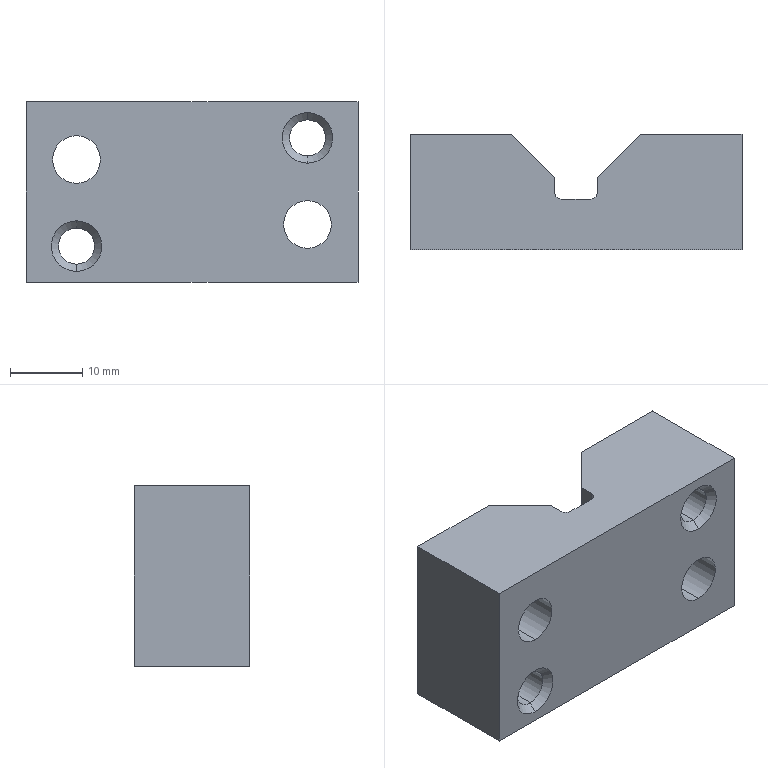Part | SolidWorks | features Chamfer 4, Cut 3, Fillet 2, Extrusion 1 | 1 solid | 36 faces | box 46 x 16 x 25 mm | volume 13455 mm3 | cylinder 14 | plane 14 | cone 8 | commonest cylinder face diameters 5 x4 6.6 x4 12 x4 2 x2
STEP:
#1=CARTESIAN_POINT('',(-16.,-15.,7.5));
#2=VERTEX_POINT('',#1);
#3=CARTESIAN_POINT('',(-16.,-15.,2.5));
#4=VERTEX_POINT('',#3);
#5=CARTESIAN_POINT('',(-16.,-15.,5.));
#6=DIRECTION('',(0.,-1.,0.));
#7=DIRECTION('',(0.,0.,1.));
#8=AXIS2_PLACEMENT_3D('',#5,#6,#7);
#9=CIRCLE('',#8,2.5);
#10=EDGE_CURVE('',#2,#4,#9,.T.);
#11=ORIENTED_EDGE('',*,*,#10,.F.);
#12=CARTESIAN_POINT('',(-16.,-16.,8.5));
#13=VERTEX_POINT('',#12);
#14=CARTESIAN_POINT('',(-16.,-16.,8.5));
#15=DIRECTION('',(0.,-0.7071,0.7071));
#16=VECTOR('',#15,1000.);
#17=LINE('',#14,#16);
#18=EDGE_CURVE('',#2,#13,#17,.T.);
#19=ORIENTED_EDGE('',*,*,#18,.T.);
#20=CARTESIAN_POINT('',(-16.,-16.,1.5));
#21=VERTEX_POINT('',#20);
#22=CARTESIAN_POINT('',(-16.,-16.,5.));
#23=DIRECTION('',(0.,1.,0.));
#24=DIRECTION('',(0.,0.,1.));
#25=AXIS2_PLACEMENT_3D('',#22,#23,#24);
#26=CIRCLE('',#25,3.5);
#27=EDGE_CURVE('',#21,#13,#26,.T.);
#28=ORIENTED_EDGE('',*,*,#27,.F.);
#29=CARTESIAN_POINT('',(-16.,-16.,1.5));
#30=DIRECTION('',(0.,-0.7071,-0.7071));
#31=VECTOR('',#30,1000.);
#32=LINE('',#29,#31);
#33=EDGE_CURVE('',#4,#21,#32,.T.);
#34=ORIENTED_EDGE('',*,*,#33,.F.);
#35=EDGE_LOOP('',(#11,#19,#28,#34));
#36=FACE_OUTER_BOUND('',#35,.T.);
#37=CARTESIAN_POINT('',(-16.,-16.,5.));
#38=DIRECTION('',(0.,-1.,0.));
#39=DIRECTION('',(0.,0.,-1.));
#40=AXIS2_PLACEMENT_3D('',#37,#38,#39);
#41=CONICAL_SURFACE('',#40,3.5,0.7854);
#42=ADVANCED_FACE('',(#36),#41,.F.);
#43=CARTESIAN_POINT('',(16.,-15.,22.5));
#44=VERTEX_POINT('',#43);
#45=CARTESIAN_POINT('',(16.,-15.,17.5));
#46=VERTEX_POINT('',#45);
#47=CARTESIAN_POINT('',(16.,-15.,20.));
#48=DIRECTION('',(0.,-1.,0.));
#49=DIRECTION('',(0.,0.,1.));
#50=AXIS2_PLACEMENT_3D('',#47,#48,#49);
#51=CIRCLE('',#50,2.5);
#52=EDGE_CURVE('',#44,#46,#51,.T.);
#53=ORIENTED_EDGE('',*,*,#52,.F.);
#54=CARTESIAN_POINT('',(16.,-16.,23.5));
#55=VERTEX_POINT('',#54);
#56=CARTESIAN_POINT('',(16.,-16.,23.5));
#57=DIRECTION('',(0.,-0.7071,0.7071));
#58=VECTOR('',#57,1000.);
#59=LINE('',#56,#58);
#60=EDGE_CURVE('',#44,#55,#59,.T.);
#61=ORIENTED_EDGE('',*,*,#60,.T.);
#62=CARTESIAN_POINT('',(16.,-16.,16.5));
#63=VERTEX_POINT('',#62);
#64=CARTESIAN_POINT('',(16.,-16.,20.));
#65=DIRECTION('',(0.,1.,0.));
#66=DIRECTION('',(0.,0.,1.));
#67=AXIS2_PLACEMENT_3D('',#64,#65,#66);
#68=CIRCLE('',#67,3.5);
#69=EDGE_CURVE('',#63,#55,#68,.T.);
#70=ORIENTED_EDGE('',*,*,#69,.F.);
#71=CARTESIAN_POINT('',(16.,-16.,16.5));
#72=DIRECTION('',(0.,-0.7071,-0.7071));
#73=VECTOR('',#72,1000.);
#74=LINE('',#71,#73);
#75=EDGE_CURVE('',#46,#63,#74,.T.);
#76=ORIENTED_EDGE('',*,*,#75,.F.);
#77=EDGE_LOOP('',(#53,#61,#70,#76));
#78=FACE_OUTER_BOUND('',#77,.T.);
#79=CARTESIAN_POINT('',(16.,-16.,20.));
#80=DIRECTION('',(0.,-1.,0.));
#81=DIRECTION('',(0.,0.,-1.));
#82=AXIS2_PLACEMENT_3D('',#79,#80,#81);
#83=CONICAL_SURFACE('',#82,3.5,0.7854);
#84=ADVANCED_FACE('',(#78),#83,.F.);
#85=CARTESIAN_POINT('',(-16.,-1.,2.5));
#86=VERTEX_POINT('',#85);
#87=CARTESIAN_POINT('',(-16.,-1.,7.5));
#88=VERTEX_POINT('',#87);
#89=CARTESIAN_POINT('',(-16.,-1.,5.));
#90=DIRECTION('',(0.,1.,0.));
#91=DIRECTION('',(0.,0.,-1.));
#92=AXIS2_PLACEMENT_3D('',#89,#90,#91);
#93=CIRCLE('',#92,2.5);
#94=EDGE_CURVE('',#86,#88,#93,.T.);
#95=ORIENTED_EDGE('',*,*,#94,.F.);
#96=CARTESIAN_POINT('',(-16.,0.,1.5));
#97=VERTEX_POINT('',#96);
#98=CARTESIAN_POINT('',(-16.,-1.,2.5));
#99=DIRECTION('',(0.,0.7071,-0.7071));
#100=VECTOR('',#99,1000.);
#101=LINE('',#98,#100);
#102=EDGE_CURVE('',#86,#97,#101,.T.);
#103=ORIENTED_EDGE('',*,*,#102,.T.);
#104=CARTESIAN_POINT('',(-16.,0.,8.5));
#105=VERTEX_POINT('',#104);
#106=CARTESIAN_POINT('',(-16.,0.,5.));
#107=DIRECTION('',(0.,-1.,0.));
#108=DIRECTION('',(1.,0.,0.));
#109=AXIS2_PLACEMENT_3D('',#106,#107,#108);
#110=CIRCLE('',#109,3.5);
#111=EDGE_CURVE('',#105,#97,#110,.T.);
#112=ORIENTED_EDGE('',*,*,#111,.F.);
#113=CARTESIAN_POINT('',(-16.,-1.,7.5));
#114=DIRECTION('',(0.,0.7071,0.7071));
#115=VECTOR('',#114,1000.);
#116=LINE('',#113,#115);
#117=EDGE_CURVE('',#88,#105,#116,.T.);
#118=ORIENTED_EDGE('',*,*,#117,.F.);
#119=EDGE_LOOP('',(#95,#103,#112,#118));
#120=FACE_OUTER_BOUND('',#119,.T.);
#121=CARTESIAN_POINT('',(-16.,-1.,5.));
#122=DIRECTION('',(0.,1.,0.));
#123=DIRECTION('',(0.,0.,1.));
#124=AXIS2_PLACEMENT_3D('',#121,#122,#123);
#125=CONICAL_SURFACE('',#124,2.5,0.7854);
#126=ADVANCED_FACE('',(#120),#125,.F.);
#127=CARTESIAN_POINT('',(16.,-1.,17.5));
#128=VERTEX_POINT('',#127);
#129=CARTESIAN_POINT('',(16.,-1.,22.5));
#130=VERTEX_POINT('',#129);
#131=CARTESIAN_POINT('',(16.,-1.,20.));
#132=DIRECTION('',(0.,1.,0.));
#133=DIRECTION('',(0.,0.,-1.));
#134=AXIS2_PLACEMENT_3D('',#131,#132,#133);
#135=CIRCLE('',#134,2.5);
#136=EDGE_CURVE('',#128,#130,#135,.T.);
#137=ORIENTED_EDGE('',*,*,#136,.F.);
#138=CARTESIAN_POINT('',(16.,0.,16.5));
#139=VERTEX_POINT('',#138);
#140=CARTESIAN_POINT('',(16.,-1.,17.5));
#141=DIRECTION('',(0.,0.7071,-0.7071));
#142=VECTOR('',#141,1000.);
#143=LINE('',#140,#142);
#144=EDGE_CURVE('',#128,#139,#143,.T.);
#145=ORIENTED_EDGE('',*,*,#144,.T.);
#146=CARTESIAN_POINT('',(16.,0.,23.5));
#147=VERTEX_POINT('',#146);
#148=CARTESIAN_POINT('',(16.,0.,20.));
#149=DIRECTION('',(0.,-1.,0.));
#150=DIRECTION('',(1.,0.,0.));
#151=AXIS2_PLACEMENT_3D('',#148,#149,#150);
#152=CIRCLE('',#151,3.5);
#153=EDGE_CURVE('',#147,#139,#152,.T.);
#154=ORIENTED_EDGE('',*,*,#153,.F.);
#155=CARTESIAN_POINT('',(16.,-1.,22.5));
#156=DIRECTION('',(0.,0.7071,0.7071));
#157=VECTOR('',#156,1000.);
#158=LINE('',#155,#157);
#159=EDGE_CURVE('',#130,#147,#158,.T.);
#160=ORIENTED_EDGE('',*,*,#159,.F.);
#161=EDGE_LOOP('',(#137,#145,#154,#160));
#162=FACE_OUTER_BOUND('',#161,.T.);
#163=CARTESIAN_POINT('',(16.,-1.,20.));
#164=DIRECTION('',(0.,1.,0.));
#165=DIRECTION('',(0.,0.,1.));
#166=AXIS2_PLACEMENT_3D('',#163,#164,#165);
#167=CONICAL_SURFACE('',#166,2.5,0.7854);
#168=ADVANCED_FACE('',(#162),#167,.F.);
#169=CARTESIAN_POINT('',(16.,-6.,2.));
#170=VERTEX_POINT('',#169);
#171=CARTESIAN_POINT('',(16.,-6.,14.));
#172=VERTEX_POINT('',#171);
#173=CARTESIAN_POINT('',(16.,-6.,8.));
#174=DIRECTION('',(0.,1.,0.));
#175=DIRECTION('',(0.,0.,1.));
#176=AXIS2_PLACEMENT_3D('',#173,#174,#175);
#177=CIRCLE('',#176,6.);
#178=EDGE_CURVE('',#170,#172,#177,.T.);
#179=ORIENTED_EDGE('',*,*,#178,.F.);
#180=CARTESIAN_POINT('',(16.,0.,2.));
#181=VERTEX_POINT('',#180);
#182=CARTESIAN_POINT('',(16.,-6.,2.));
#183=DIRECTION('',(0.,1.,0.));
#184=VECTOR('',#183,1000.);
#185=LINE('',#182,#184);
#186=EDGE_CURVE('',#170,#181,#185,.T.);
#187=ORIENTED_EDGE('',*,*,#186,.T.);
#188=CARTESIAN_POINT('',(16.,0.,14.));
#189=VERTEX_POINT('',#188);
#190=CARTESIAN_POINT('',(16.,0.,8.));
#191=DIRECTION('',(0.,1.,0.));
#192=DIRECTION('',(0.,0.,1.));
#193=AXIS2_PLACEMENT_3D('',#190,#191,#192);
#194=CIRCLE('',#193,6.);
#195=EDGE_CURVE('',#181,#189,#194,.T.);
#196=ORIENTED_EDGE('',*,*,#195,.T.);
#197=CARTESIAN_POINT('',(16.,-6.,14.));
#198=DIRECTION('',(0.,1.,0.));
#199=VECTOR('',#198,1000.);
#200=LINE('',#197,#199);
#201=EDGE_CURVE('',#172,#189,#200,.T.);
#202=ORIENTED_EDGE('',*,*,#201,.F.);
#203=EDGE_LOOP('',(#179,#187,#196,#202));
#204=FACE_OUTER_BOUND('',#203,.T.);
#205=CARTESIAN_POINT('',(16.,-6.,8.));
#206=DIRECTION('',(0.,1.,0.));
#207=DIRECTION('',(0.,0.,1.));
#208=AXIS2_PLACEMENT_3D('',#205,#206,#207);
#209=CYLINDRICAL_SURFACE('',#208,6.);
#210=ADVANCED_FACE('',(#204),#209,.F.);
#211=CARTESIAN_POINT('',(-16.,-6.,11.));
#212=VERTEX_POINT('',#211);
#213=CARTESIAN_POINT('',(-16.,-6.,23.));
#214=VERTEX_POINT('',#213);
#215=CARTESIAN_POINT('',(-16.,-6.,17.));
#216=DIRECTION('',(0.,1.,0.));
#217=DIRECTION('',(0.,0.,1.));
#218=AXIS2_PLACEMENT_3D('',#215,#216,#217);
#219=CIRCLE('',#218,6.);
#220=EDGE_CURVE('',#212,#214,#219,.T.);
#221=ORIENTED_EDGE('',*,*,#220,.F.);
#222=CARTESIAN_POINT('',(-16.,0.,11.));
#223=VERTEX_POINT('',#222);
#224=CARTESIAN_POINT('',(-16.,-6.,11.));
#225=DIRECTION('',(0.,1.,0.));
#226=VECTOR('',#225,1000.);
#227=LINE('',#224,#226);
#228=EDGE_CURVE('',#212,#223,#227,.T.);
#229=ORIENTED_EDGE('',*,*,#228,.T.);
#230=CARTESIAN_POINT('',(-16.,0.,23.));
#231=VERTEX_POINT('',#230);
#232=CARTESIAN_POINT('',(-16.,0.,17.));
#233=DIRECTION('',(0.,1.,0.));
#234=DIRECTION('',(0.,0.,1.));
#235=AXIS2_PLACEMENT_3D('',#232,#233,#234);
#236=CIRCLE('',#235,6.);
#237=EDGE_CURVE('',#223,#231,#236,.T.);
#238=ORIENTED_EDGE('',*,*,#237,.T.);
#239=CARTESIAN_POINT('',(-16.,-6.,23.));
#240=DIRECTION('',(0.,1.,0.));
#241=VECTOR('',#240,1000.);
#242=LINE('',#239,#241);
#243=EDGE_CURVE('',#214,#231,#242,.T.);
#244=ORIENTED_EDGE('',*,*,#243,.F.);
#245=EDGE_LOOP('',(#221,#229,#238,#244));
#246=FACE_OUTER_BOUND('',#245,.T.);
#247=CARTESIAN_POINT('',(-16.,-6.,17.));
#248=DIRECTION('',(0.,1.,0.));
#249=DIRECTION('',(0.,0.,1.));
#250=AXIS2_PLACEMENT_3D('',#247,#248,#249);
#251=CYLINDRICAL_SURFACE('',#250,6.);
#252=ADVANCED_FACE('',(#246),#251,.F.);
#253=ORIENTED_EDGE('',*,*,#52,.T.);
#254=CARTESIAN_POINT('',(16.,-16.,17.5));
#255=DIRECTION('',(0.,1.,0.));
#256=VECTOR('',#255,1000.);
#257=LINE('',#254,#256);
#258=EDGE_CURVE('',#46,#128,#257,.T.);
#259=ORIENTED_EDGE('',*,*,#258,.T.);
#260=ORIENTED_EDGE('',*,*,#136,.T.);
#261=CARTESIAN_POINT('',(16.,-16.,22.5));
#262=DIRECTION('',(0.,1.,0.));
#263=VECTOR('',#262,1000.);
#264=LINE('',#261,#263);
#265=EDGE_CURVE('',#44,#130,#264,.T.);
#266=ORIENTED_EDGE('',*,*,#265,.F.);
#267=EDGE_LOOP('',(#253,#259,#260,#266));
#268=FACE_OUTER_BOUND('',#267,.T.);
#269=CARTESIAN_POINT('',(16.,-16.,20.));
#270=DIRECTION('',(0.,1.,0.));
#271=DIRECTION('',(0.,0.,1.));
#272=AXIS2_PLACEMENT_3D('',#269,#270,#271);
#273=CYLINDRICAL_SURFACE('',#272,2.5);
#274=ADVANCED_FACE('',(#268),#273,.F.);
#275=ORIENTED_EDGE('',*,*,#10,.T.);
#276=CARTESIAN_POINT('',(-16.,-16.,2.5));
#277=DIRECTION('',(0.,1.,0.));
#278=VECTOR('',#277,1000.);
#279=LINE('',#276,#278);
#280=EDGE_CURVE('',#4,#86,#279,.T.);
#281=ORIENTED_EDGE('',*,*,#280,.T.);
#282=ORIENTED_EDGE('',*,*,#94,.T.);
#283=CARTESIAN_POINT('',(-16.,-16.,7.5));
#284=DIRECTION('',(0.,1.,0.));
#285=VECTOR('',#284,1000.);
#286=LINE('',#283,#285);
#287=EDGE_CURVE('',#2,#88,#286,.T.);
#288=ORIENTED_EDGE('',*,*,#287,.F.);
#289=EDGE_LOOP('',(#275,#281,#282,#288));
#290=FACE_OUTER_BOUND('',#289,.T.);
#291=CARTESIAN_POINT('',(-16.,-16.,5.));
#292=DIRECTION('',(0.,1.,0.));
#293=DIRECTION('',(0.,0.,1.));
#294=AXIS2_PLACEMENT_3D('',#291,#292,#293);
#295=CYLINDRICAL_SURFACE('',#294,2.5);
#296=ADVANCED_FACE('',(#290),#295,.F.);
#297=CARTESIAN_POINT('',(-16.,-16.,13.7));
#298=VERTEX_POINT('',#297);
#299=CARTESIAN_POINT('',(-16.,-16.,20.3));
#300=VERTEX_POINT('',#299);
#301=CARTESIAN_POINT('',(-16.,-16.,17.));
#302=DIRECTION('',(0.,1.,0.));
#303=DIRECTION('',(0.,0.,1.));
#304=AXIS2_PLACEMENT_3D('',#301,#302,#303);
#305=CIRCLE('',#304,3.3);
#306=EDGE_CURVE('',#298,#300,#305,.T.);
#307=ORIENTED_EDGE('',*,*,#306,.F.);
#308=CARTESIAN_POINT('',(-16.,-6.,13.7));
#309=VERTEX_POINT('',#308);
#310=CARTESIAN_POINT('',(-16.,-16.,13.7));
#311=DIRECTION('',(0.,1.,0.));
#312=VECTOR('',#311,1000.);
#313=LINE('',#310,#312);
#314=EDGE_CURVE('',#298,#309,#313,.T.);
#315=ORIENTED_EDGE('',*,*,#314,.T.);
#316=CARTESIAN_POINT('',(-16.,-6.,20.3));
#317=VERTEX_POINT('',#316);
#318=CARTESIAN_POINT('',(-16.,-6.,17.));
#319=DIRECTION('',(0.,-1.,0.));
#320=DIRECTION('',(0.,0.,1.));
#321=AXIS2_PLACEMENT_3D('',#318,#319,#320);
#322=CIRCLE('',#321,3.3);
#323=EDGE_CURVE('',#317,#309,#322,.T.);
#324=ORIENTED_EDGE('',*,*,#323,.F.);
#325=CARTESIAN_POINT('',(-16.,-16.,20.3));
#326=DIRECTION('',(0.,1.,0.));
#327=VECTOR('',#326,1000.);
#328=LINE('',#325,#327);
#329=EDGE_CURVE('',#300,#317,#328,.T.);
#330=ORIENTED_EDGE('',*,*,#329,.F.);
#331=EDGE_LOOP('',(#307,#315,#324,#330));
#332=FACE_OUTER_BOUND('',#331,.T.);
#333=CARTESIAN_POINT('',(-16.,-16.,17.));
#334=DIRECTION('',(0.,1.,0.));
#335=DIRECTION('',(0.,0.,1.));
#336=AXIS2_PLACEMENT_3D('',#333,#334,#335);
#337=CYLINDRICAL_SURFACE('',#336,3.3);
#338=ADVANCED_FACE('',(#332),#337,.F.);
#339=CARTESIAN_POINT('',(16.,-16.,4.7));
#340=VERTEX_POINT('',#339);
#341=CARTESIAN_POINT('',(16.,-16.,11.3));
#342=VERTEX_POINT('',#341);
#343=CARTESIAN_POINT('',(16.,-16.,8.));
#344=DIRECTION('',(0.,1.,0.));
#345=DIRECTION('',(0.,0.,1.));
#346=AXIS2_PLACEMENT_3D('',#343,#344,#345);
#347=CIRCLE('',#346,3.3);
#348=EDGE_CURVE('',#340,#342,#347,.T.);
#349=ORIENTED_EDGE('',*,*,#348,.F.);
#350=CARTESIAN_POINT('',(16.,-6.,4.7));
#351=VERTEX_POINT('',#350);
#352=CARTESIAN_POINT('',(16.,-16.,4.7));
#353=DIRECTION('',(0.,1.,0.));
#354=VECTOR('',#353,1000.);
#355=LINE('',#352,#354);
#356=EDGE_CURVE('',#340,#351,#355,.T.);
#357=ORIENTED_EDGE('',*,*,#356,.T.);
#358=CARTESIAN_POINT('',(16.,-6.,11.3));
#359=VERTEX_POINT('',#358);
#360=CARTESIAN_POINT('',(16.,-6.,8.));
#361=DIRECTION('',(0.,-1.,0.));
#362=DIRECTION('',(0.,0.,1.));
#363=AXIS2_PLACEMENT_3D('',#360,#361,#362);
#364=CIRCLE('',#363,3.3);
#365=EDGE_CURVE('',#359,#351,#364,.T.);
#366=ORIENTED_EDGE('',*,*,#365,.F.);
#367=CARTESIAN_POINT('',(16.,-16.,11.3));
#368=DIRECTION('',(0.,1.,0.));
#369=VECTOR('',#368,1000.);
#370=LINE('',#367,#369);
#371=EDGE_CURVE('',#342,#359,#370,.T.);
#372=ORIENTED_EDGE('',*,*,#371,.F.);
#373=EDGE_LOOP('',(#349,#357,#366,#372));
#374=FACE_OUTER_BOUND('',#373,.T.);
#375=CARTESIAN_POINT('',(16.,-16.,8.));
#376=DIRECTION('',(0.,1.,0.));
#377=DIRECTION('',(0.,0.,1.));
#378=AXIS2_PLACEMENT_3D('',#375,#376,#377);
#379=CYLINDRICAL_SURFACE('',#378,3.3);
#380=ADVANCED_FACE('',(#374),#379,.F.);
#381=ORIENTED_EDGE('',*,*,#356,.F.);
#382=CARTESIAN_POINT('',(16.,-16.,8.));
#383=DIRECTION('',(0.,1.,0.));
#384=DIRECTION('',(0.,0.,1.));
#385=AXIS2_PLACEMENT_3D('',#382,#383,#384);
#386=CIRCLE('',#385,3.3);
#387=EDGE_CURVE('',#342,#340,#386,.T.);
#388=ORIENTED_EDGE('',*,*,#387,.F.);
#389=ORIENTED_EDGE('',*,*,#371,.T.);
#390=CARTESIAN_POINT('',(16.,-6.,8.));
#391=DIRECTION('',(0.,-1.,0.));
#392=DIRECTION('',(0.,0.,1.));
#393=AXIS2_PLACEMENT_3D('',#390,#391,#392);
#394=CIRCLE('',#393,3.3);
#395=EDGE_CURVE('',#351,#359,#394,.T.);
#396=ORIENTED_EDGE('',*,*,#395,.F.);
#397=EDGE_LOOP('',(#381,#388,#389,#396));
#398=FACE_OUTER_BOUND('',#397,.T.);
#399=CARTESIAN_POINT('',(16.,-16.,8.));
#400=DIRECTION('',(0.,1.,0.));
#401=DIRECTION('',(0.,0.,1.));
#402=AXIS2_PLACEMENT_3D('',#399,#400,#401);
#403=CYLINDRICAL_SURFACE('',#402,3.3);
#404=ADVANCED_FACE('',(#398),#403,.F.);
#405=ORIENTED_EDGE('',*,*,#314,.F.);
#406=CARTESIAN_POINT('',(-16.,-16.,17.));
#407=DIRECTION('',(0.,1.,0.));
#408=DIRECTION('',(0.,0.,1.));
#409=AXIS2_PLACEMENT_3D('',#406,#407,#408);
#410=CIRCLE('',#409,3.3);
#411=EDGE_CURVE('',#300,#298,#410,.T.);
#412=ORIENTED_EDGE('',*,*,#411,.F.);
#413=ORIENTED_EDGE('',*,*,#329,.T.);
#414=CARTESIAN_POINT('',(-16.,-6.,17.));
#415=DIRECTION('',(0.,-1.,0.));
#416=DIRECTION('',(0.,0.,1.));
#417=AXIS2_PLACEMENT_3D('',#414,#415,#416);
#418=CIRCLE('',#417,3.3);
#419=EDGE_CURVE('',#309,#317,#418,.T.);
#420=ORIENTED_EDGE('',*,*,#419,.F.);
#421=EDGE_LOOP('',(#405,#412,#413,#420));
#422=FACE_OUTER_BOUND('',#421,.T.);
#423=CARTESIAN_POINT('',(-16.,-16.,17.));
#424=DIRECTION('',(0.,1.,0.));
#425=DIRECTION('',(0.,0.,1.));
#426=AXIS2_PLACEMENT_3D('',#423,#424,#425);
#427=CYLINDRICAL_SURFACE('',#426,3.3);
#428=ADVANCED_FACE('',(#422),#427,.F.);
#429=ORIENTED_EDGE('',*,*,#111,.T.);
#430=CARTESIAN_POINT('',(-16.,0.,5.));
#431=DIRECTION('',(0.,-1.,0.));
#432=DIRECTION('',(1.,0.,0.));
#433=AXIS2_PLACEMENT_3D('',#430,#431,#432);
#434=CIRCLE('',#433,3.5);
#435=EDGE_CURVE('',#97,#105,#434,.T.);
#436=ORIENTED_EDGE('',*,*,#435,.T.);
#437=EDGE_LOOP('',(#429,#436));
#438=FACE_BOUND('',#437,.T.);
#439=CARTESIAN_POINT('',(-16.,0.,17.));
#440=DIRECTION('',(0.,1.,0.));
#441=DIRECTION('',(0.,0.,1.));
#442=AXIS2_PLACEMENT_3D('',#439,#440,#441);
#443=CIRCLE('',#442,6.);
#444=EDGE_CURVE('',#231,#223,#443,.T.);
#445=ORIENTED_EDGE('',*,*,#444,.F.);
#446=ORIENTED_EDGE('',*,*,#237,.F.);
#447=EDGE_LOOP('',(#445,#446));
#448=FACE_BOUND('',#447,.T.);
#449=CARTESIAN_POINT('',(-9.,0.,25.));
#450=VERTEX_POINT('',#449);
#451=CARTESIAN_POINT('',(-23.,0.,25.));
#452=VERTEX_POINT('',#451);
#453=CARTESIAN_POINT('',(-23.,0.,25.));
#454=DIRECTION('',(-1.,0.,0.));
#455=VECTOR('',#454,1000.);
#456=LINE('',#453,#455);
#457=EDGE_CURVE('',#450,#452,#456,.T.);
#458=ORIENTED_EDGE('',*,*,#457,.F.);
#459=CARTESIAN_POINT('',(-9.,0.,0.));
#460=VERTEX_POINT('',#459);
#461=CARTESIAN_POINT('',(-9.,0.,0.));
#462=DIRECTION('',(0.,0.,1.));
#463=VECTOR('',#462,1000.);
#464=LINE('',#461,#463);
#465=EDGE_CURVE('',#460,#450,#464,.T.);
#466=ORIENTED_EDGE('',*,*,#465,.F.);
#467=CARTESIAN_POINT('',(-23.,0.,0.));
#468=VERTEX_POINT('',#467);
#469=CARTESIAN_POINT('',(-23.,0.,0.));
#470=DIRECTION('',(-1.,0.,0.));
#471=VECTOR('',#470,1000.);
#472=LINE('',#469,#471);
#473=EDGE_CURVE('',#460,#468,#472,.T.);
#474=ORIENTED_EDGE('',*,*,#473,.T.);
#475=CARTESIAN_POINT('',(-23.,0.,25.));
#476=DIRECTION('',(0.,0.,-1.));
#477=VECTOR('',#476,1000.);
#478=LINE('',#475,#477);
#479=EDGE_CURVE('',#452,#468,#478,.T.);
#480=ORIENTED_EDGE('',*,*,#479,.F.);
#481=EDGE_LOOP('',(#458,#466,#474,#480));
#482=FACE_OUTER_BOUND('',#481,.T.);
#483=CARTESIAN_POINT('',(-23.,0.,25.));
#484=DIRECTION('',(0.,-1.,0.));
#485=DIRECTION('',(1.,0.,0.));
#486=AXIS2_PLACEMENT_3D('',#483,#484,#485);
#487=PLANE('',#486);
#488=ADVANCED_FACE('',(#438,#448,#482),#487,.F.);
#489=CARTESIAN_POINT('',(-23.,-16.,0.));
#490=VERTEX_POINT('',#489);
#491=CARTESIAN_POINT('',(-23.,0.,0.));
#492=DIRECTION('',(0.,-1.,0.));
#493=VECTOR('',#492,1000.);
#494=LINE('',#491,#493);
#495=EDGE_CURVE('',#468,#490,#494,.T.);
#496=ORIENTED_EDGE('',*,*,#495,.T.);
#497=CARTESIAN_POINT('',(-23.,-16.,25.));
#498=VERTEX_POINT('',#497);
#499=CARTESIAN_POINT('',(-23.,-16.,25.));
#500=DIRECTION('',(0.,0.,-1.));
#501=VECTOR('',#500,1000.);
#502=LINE('',#499,#501);
#503=EDGE_CURVE('',#498,#490,#502,.T.);
#504=ORIENTED_EDGE('',*,*,#503,.F.);
#505=CARTESIAN_POINT('',(-23.,0.,25.));
#506=DIRECTION('',(0.,-1.,0.));
#507=VECTOR('',#506,1000.);
#508=LINE('',#505,#507);
#509=EDGE_CURVE('',#452,#498,#508,.T.);
#510=ORIENTED_EDGE('',*,*,#509,.F.);
#511=ORIENTED_EDGE('',*,*,#479,.T.);
#512=EDGE_LOOP('',(#496,#504,#510,#511));
#513=FACE_OUTER_BOUND('',#512,.T.);
#514=CARTESIAN_POINT('',(-23.,0.,25.));
#515=DIRECTION('',(1.,0.,0.));
#516=DIRECTION('',(0.,1.,0.));
#517=AXIS2_PLACEMENT_3D('',#514,#515,#516);
#518=PLANE('',#517);
#519=ADVANCED_FACE('',(#513),#518,.F.);
#520=ORIENTED_EDGE('',*,*,#27,.T.);
#521=CARTESIAN_POINT('',(-16.,-16.,5.));
#522=DIRECTION('',(0.,1.,0.));
#523=DIRECTION('',(0.,0.,1.));
#524=AXIS2_PLACEMENT_3D('',#521,#522,#523);
#525=CIRCLE('',#524,3.5);
#526=EDGE_CURVE('',#13,#21,#525,.T.);
#527=ORIENTED_EDGE('',*,*,#526,.T.);
#528=EDGE_LOOP('',(#520,#527));
#529=FACE_BOUND('',#528,.T.);
#530=ORIENTED_EDGE('',*,*,#69,.T.);
#531=CARTESIAN_POINT('',(16.,-16.,20.));
#532=DIRECTION('',(0.,1.,0.));
#533=DIRECTION('',(0.,0.,1.));
#534=AXIS2_PLACEMENT_3D('',#531,#532,#533);
#535=CIRCLE('',#534,3.5);
#536=EDGE_CURVE('',#55,#63,#535,.T.);
#537=ORIENTED_EDGE('',*,*,#536,.T.);
#538=EDGE_LOOP('',(#530,#537));
#539=FACE_BOUND('',#538,.T.);
#540=ORIENTED_EDGE('',*,*,#387,.T.);
#541=ORIENTED_EDGE('',*,*,#348,.T.);
#542=EDGE_LOOP('',(#540,#541));
#543=FACE_BOUND('',#542,.T.);
#544=ORIENTED_EDGE('',*,*,#411,.T.);
#545=ORIENTED_EDGE('',*,*,#306,.T.);
#546=EDGE_LOOP('',(#544,#545));
#547=FACE_BOUND('',#546,.T.);
#548=CARTESIAN_POINT('',(23.,-16.,0.));
#549=VERTEX_POINT('',#548);
#550=CARTESIAN_POINT('',(-23.,-16.,0.));
#551=DIRECTION('',(1.,0.,0.));
#552=VECTOR('',#551,1000.);
#553=LINE('',#550,#552);
#554=EDGE_CURVE('',#490,#549,#553,.T.);
#555=ORIENTED_EDGE('',*,*,#554,.T.);
#556=CARTESIAN_POINT('',(23.,-16.,25.));
#557=VERTEX_POINT('',#556);
#558=CARTESIAN_POINT('',(23.,-16.,25.));
#559=DIRECTION('',(0.,0.,-1.));
#560=VECTOR('',#559,1000.);
#561=LINE('',#558,#560);
#562=EDGE_CURVE('',#557,#549,#561,.T.);
#563=ORIENTED_EDGE('',*,*,#562,.F.);
#564=CARTESIAN_POINT('',(-23.,-16.,25.));
#565=DIRECTION('',(1.,0.,0.));
#566=VECTOR('',#565,1000.);
#567=LINE('',#564,#566);
#568=EDGE_CURVE('',#498,#557,#567,.T.);
#569=ORIENTED_EDGE('',*,*,#568,.F.);
#570=ORIENTED_EDGE('',*,*,#503,.T.);
#571=EDGE_LOOP('',(#555,#563,#569,#570));
#572=FACE_OUTER_BOUND('',#571,.T.);
#573=CARTESIAN_POINT('',(-23.,-16.,25.));
#574=DIRECTION('',(0.,1.,0.));
#575=DIRECTION('',(0.,0.,1.));
#576=AXIS2_PLACEMENT_3D('',#573,#574,#575);
#577=PLANE('',#576);
#578=ADVANCED_FACE('',(#529,#539,#543,#547,#572),#577,.F.);
#579=CARTESIAN_POINT('',(23.,0.,0.));
#580=VERTEX_POINT('',#579);
#581=CARTESIAN_POINT('',(23.,0.,0.));
#582=DIRECTION('',(0.,1.,0.));
#583=VECTOR('',#582,1000.);
#584=LINE('',#581,#583);
#585=EDGE_CURVE('',#549,#580,#584,.T.);
#586=ORIENTED_EDGE('',*,*,#585,.T.);
#587=CARTESIAN_POINT('',(23.,0.,25.));
#588=VERTEX_POINT('',#587);
#589=CARTESIAN_POINT('',(23.,0.,25.));
#590=DIRECTION('',(0.,0.,-1.));
#591=VECTOR('',#590,1000.);
#592=LINE('',#589,#591);
#593=EDGE_CURVE('',#588,#580,#592,.T.);
#594=ORIENTED_EDGE('',*,*,#593,.F.);
#595=CARTESIAN_POINT('',(23.,0.,25.));
#596=DIRECTION('',(0.,1.,0.));
#597=VECTOR('',#596,1000.);
#598=LINE('',#595,#597);
#599=EDGE_CURVE('',#557,#588,#598,.T.);
#600=ORIENTED_EDGE('',*,*,#599,.F.);
#601=ORIENTED_EDGE('',*,*,#562,.T.);
#602=EDGE_LOOP('',(#586,#594,#600,#601));
#603=FACE_OUTER_BOUND('',#602,.T.);
#604=CARTESIAN_POINT('',(23.,0.,25.));
#605=DIRECTION('',(-1.,0.,0.));
#606=DIRECTION('',(0.,-1.,0.));
#607=AXIS2_PLACEMENT_3D('',#604,#605,#606);
#608=PLANE('',#607);
#609=ADVANCED_FACE('',(#603),#608,.F.);
#610=ORIENTED_EDGE('',*,*,#153,.T.);
#611=CARTESIAN_POINT('',(16.,0.,20.));
#612=DIRECTION('',(0.,-1.,0.));
#613=DIRECTION('',(1.,0.,0.));
#614=AXIS2_PLACEMENT_3D('',#611,#612,#613);
#615=CIRCLE('',#614,3.5);
#616=EDGE_CURVE('',#139,#147,#615,.T.);
#617=ORIENTED_EDGE('',*,*,#616,.T.);
#618=EDGE_LOOP('',(#610,#617));
#619=FACE_BOUND('',#618,.T.);
#620=CARTESIAN_POINT('',(16.,0.,8.));
#621=DIRECTION('',(0.,1.,0.));
#622=DIRECTION('',(0.,0.,1.));
#623=AXIS2_PLACEMENT_3D('',#620,#621,#622);
#624=CIRCLE('',#623,6.);
#625=EDGE_CURVE('',#189,#181,#624,.T.);
#626=ORIENTED_EDGE('',*,*,#625,.F.);
#627=ORIENTED_EDGE('',*,*,#195,.F.);
#628=EDGE_LOOP('',(#626,#627));
#629=FACE_BOUND('',#628,.T.);
#630=CARTESIAN_POINT('',(9.,0.,0.));
#631=VERTEX_POINT('',#630);
#632=CARTESIAN_POINT('',(-23.,0.,0.));
#633=DIRECTION('',(-1.,0.,0.));
#634=VECTOR('',#633,1000.);
#635=LINE('',#632,#634);
#636=EDGE_CURVE('',#580,#631,#635,.T.);
#637=ORIENTED_EDGE('',*,*,#636,.T.);
#638=CARTESIAN_POINT('',(9.,0.,25.));
#639=VERTEX_POINT('',#638);
#640=CARTESIAN_POINT('',(9.,0.,0.));
#641=DIRECTION('',(0.,0.,1.));
#642=VECTOR('',#641,1000.);
#643=LINE('',#640,#642);
#644=EDGE_CURVE('',#631,#639,#643,.T.);
#645=ORIENTED_EDGE('',*,*,#644,.T.);
#646=CARTESIAN_POINT('',(-23.,0.,25.));
#647=DIRECTION('',(-1.,0.,0.));
#648=VECTOR('',#647,1000.);
#649=LINE('',#646,#648);
#650=EDGE_CURVE('',#588,#639,#649,.T.);
#651=ORIENTED_EDGE('',*,*,#650,.F.);
#652=ORIENTED_EDGE('',*,*,#593,.T.);
#653=EDGE_LOOP('',(#637,#645,#651,#652));
#654=FACE_OUTER_BOUND('',#653,.T.);
#655=CARTESIAN_POINT('',(-23.,0.,25.));
#656=DIRECTION('',(0.,-1.,0.));
#657=DIRECTION('',(1.,0.,0.));
#658=AXIS2_PLACEMENT_3D('',#655,#656,#657);
#659=PLANE('',#658);
#660=ADVANCED_FACE('',(#619,#629,#654),#659,.F.);
#661=CARTESIAN_POINT('',(-3.,-6.,25.));
#662=VERTEX_POINT('',#661);
#663=CARTESIAN_POINT('',(-9.,0.,25.));
#664=DIRECTION('',(0.7071,-0.7071,0.));
#665=VECTOR('',#664,1000.);
#666=LINE('',#663,#665);
#667=EDGE_CURVE('',#450,#662,#666,.T.);
#668=ORIENTED_EDGE('',*,*,#667,.F.);
#669=ORIENTED_EDGE('',*,*,#457,.T.);
#670=ORIENTED_EDGE('',*,*,#509,.T.);
#671=ORIENTED_EDGE('',*,*,#568,.T.);
#672=ORIENTED_EDGE('',*,*,#599,.T.);
#673=ORIENTED_EDGE('',*,*,#650,.T.);
#674=CARTESIAN_POINT('',(3.,-6.,25.));
#675=VERTEX_POINT('',#674);
#676=CARTESIAN_POINT('',(9.,0.,25.));
#677=DIRECTION('',(0.7071,0.7071,0.));
#678=VECTOR('',#677,1000.);
#679=LINE('',#676,#678);
#680=EDGE_CURVE('',#675,#639,#679,.T.);
#681=ORIENTED_EDGE('',*,*,#680,.F.);
#682=CARTESIAN_POINT('',(3.,-8.,25.));
#683=VERTEX_POINT('',#682);
#684=CARTESIAN_POINT('',(3.,-6.,25.));
#685=DIRECTION('',(0.,1.,0.));
#686=VECTOR('',#685,1000.);
#687=LINE('',#684,#686);
#688=EDGE_CURVE('',#683,#675,#687,.T.);
#689=ORIENTED_EDGE('',*,*,#688,.F.);
#690=CARTESIAN_POINT('',(2.,-9.,25.));
#691=VERTEX_POINT('',#690);
#692=CARTESIAN_POINT('',(2.,-8.,25.));
#693=DIRECTION('',(0.,0.,-1.));
#694=DIRECTION('',(1.,0.,0.));
#695=AXIS2_PLACEMENT_3D('',#692,#693,#694);
#696=CIRCLE('',#695,1.);
#697=EDGE_CURVE('',#683,#691,#696,.T.);
#698=ORIENTED_EDGE('',*,*,#697,.T.);
#699=CARTESIAN_POINT('',(-2.,-9.,25.));
#700=VERTEX_POINT('',#699);
#701=CARTESIAN_POINT('',(-3.,-9.,25.));
#702=DIRECTION('',(1.,0.,0.));
#703=VECTOR('',#702,1000.);
#704=LINE('',#701,#703);
#705=EDGE_CURVE('',#700,#691,#704,.T.);
#706=ORIENTED_EDGE('',*,*,#705,.F.);
#707=CARTESIAN_POINT('',(-3.,-8.,25.));
#708=VERTEX_POINT('',#707);
#709=CARTESIAN_POINT('',(-2.,-8.,25.));
#710=DIRECTION('',(0.,0.,-1.));
#711=DIRECTION('',(1.,0.,0.));
#712=AXIS2_PLACEMENT_3D('',#709,#710,#711);
#713=CIRCLE('',#712,1.);
#714=EDGE_CURVE('',#700,#708,#713,.T.);
#715=ORIENTED_EDGE('',*,*,#714,.T.);
#716=CARTESIAN_POINT('',(-3.,-6.,25.));
#717=DIRECTION('',(0.,-1.,0.));
#718=VECTOR('',#717,1000.);
#719=LINE('',#716,#718);
#720=EDGE_CURVE('',#662,#708,#719,.T.);
#721=ORIENTED_EDGE('',*,*,#720,.F.);
#722=EDGE_LOOP('',(#668,#669,#670,#671,#672,#673,#681,#689,#698,#706,#715,#721));
#723=FACE_OUTER_BOUND('',#722,.T.);
#724=CARTESIAN_POINT('',(-23.,0.,25.));
#725=DIRECTION('',(0.,0.,1.));
#726=DIRECTION('',(1.,0.,0.));
#727=AXIS2_PLACEMENT_3D('',#724,#725,#726);
#728=PLANE('',#727);
#729=ADVANCED_FACE('',(#723),#728,.T.);
#730=ORIENTED_EDGE('',*,*,#473,.F.);
#731=CARTESIAN_POINT('',(-3.,-6.,0.));
#732=VERTEX_POINT('',#731);
#733=CARTESIAN_POINT('',(-9.,0.,0.));
#734=DIRECTION('',(0.7071,-0.7071,0.));
#735=VECTOR('',#734,1000.);
#736=LINE('',#733,#735);
#737=EDGE_CURVE('',#460,#732,#736,.T.);
#738=ORIENTED_EDGE('',*,*,#737,.T.);
#739=CARTESIAN_POINT('',(-3.,-8.,0.));
#740=VERTEX_POINT('',#739);
#741=CARTESIAN_POINT('',(-3.,-6.,0.));
#742=DIRECTION('',(0.,-1.,0.));
#743=VECTOR('',#742,1000.);
#744=LINE('',#741,#743);
#745=EDGE_CURVE('',#732,#740,#744,.T.);
#746=ORIENTED_EDGE('',*,*,#745,.T.);
#747=CARTESIAN_POINT('',(-2.,-9.,0.));
#748=VERTEX_POINT('',#747);
#749=CARTESIAN_POINT('',(-2.,-8.,0.));
#750=DIRECTION('',(0.,0.,1.));
#751=DIRECTION('',(1.,0.,0.));
#752=AXIS2_PLACEMENT_3D('',#749,#750,#751);
#753=CIRCLE('',#752,1.);
#754=EDGE_CURVE('',#740,#748,#753,.T.);
#755=ORIENTED_EDGE('',*,*,#754,.T.);
#756=CARTESIAN_POINT('',(2.,-9.,0.));
#757=VERTEX_POINT('',#756);
#758=CARTESIAN_POINT('',(-3.,-9.,0.));
#759=DIRECTION('',(1.,0.,0.));
#760=VECTOR('',#759,1000.);
#761=LINE('',#758,#760);
#762=EDGE_CURVE('',#748,#757,#761,.T.);
#763=ORIENTED_EDGE('',*,*,#762,.T.);
#764=CARTESIAN_POINT('',(3.,-8.,0.));
#765=VERTEX_POINT('',#764);
#766=CARTESIAN_POINT('',(2.,-8.,0.));
#767=DIRECTION('',(0.,0.,1.));
#768=DIRECTION('',(1.,0.,0.));
#769=AXIS2_PLACEMENT_3D('',#766,#767,#768);
#770=CIRCLE('',#769,1.);
#771=EDGE_CURVE('',#757,#765,#770,.T.);
#772=ORIENTED_EDGE('',*,*,#771,.T.);
#773=CARTESIAN_POINT('',(3.,-6.,0.));
#774=VERTEX_POINT('',#773);
#775=CARTESIAN_POINT('',(3.,-6.,0.));
#776=DIRECTION('',(0.,1.,0.));
#777=VECTOR('',#776,1000.);
#778=LINE('',#775,#777);
#779=EDGE_CURVE('',#765,#774,#778,.T.);
#780=ORIENTED_EDGE('',*,*,#779,.T.);
#781=CARTESIAN_POINT('',(9.,0.,0.));
#782=DIRECTION('',(0.7071,0.7071,0.));
#783=VECTOR('',#782,1000.);
#784=LINE('',#781,#783);
#785=EDGE_CURVE('',#774,#631,#784,.T.);
#786=ORIENTED_EDGE('',*,*,#785,.T.);
#787=ORIENTED_EDGE('',*,*,#636,.F.);
#788=ORIENTED_EDGE('',*,*,#585,.F.);
#789=ORIENTED_EDGE('',*,*,#554,.F.);
#790=ORIENTED_EDGE('',*,*,#495,.F.);
#791=EDGE_LOOP('',(#730,#738,#746,#755,#763,#772,#780,#786,#787,#788,#789,#790));
#792=FACE_OUTER_BOUND('',#791,.T.);
#793=CARTESIAN_POINT('',(-23.,0.,0.));
#794=DIRECTION('',(0.,0.,1.));
#795=DIRECTION('',(1.,0.,0.));
#796=AXIS2_PLACEMENT_3D('',#793,#794,#795);
#797=PLANE('',#796);
#798=ADVANCED_FACE('',(#792),#797,.F.);
#799=ORIENTED_EDGE('',*,*,#720,.T.);
#800=CARTESIAN_POINT('',(-3.,-8.,0.));
#801=DIRECTION('',(0.,0.,-1.));
#802=VECTOR('',#801,1000.);
#803=LINE('',#800,#802);
#804=EDGE_CURVE('',#708,#740,#803,.T.);
#805=ORIENTED_EDGE('',*,*,#804,.T.);
#806=ORIENTED_EDGE('',*,*,#745,.F.);
#807=CARTESIAN_POINT('',(-3.,-6.,0.));
#808=DIRECTION('',(0.,0.,1.));
#809=VECTOR('',#808,1000.);
#810=LINE('',#807,#809);
#811=EDGE_CURVE('',#732,#662,#810,.T.);
#812=ORIENTED_EDGE('',*,*,#811,.T.);
#813=EDGE_LOOP('',(#799,#805,#806,#812));
#814=FACE_OUTER_BOUND('',#813,.T.);
#815=CARTESIAN_POINT('',(-3.,-6.,0.));
#816=DIRECTION('',(-1.,0.,0.));
#817=DIRECTION('',(0.,0.,1.));
#818=AXIS2_PLACEMENT_3D('',#815,#816,#817);
#819=PLANE('',#818);
#820=ADVANCED_FACE('',(#814),#819,.F.);
#821=ORIENTED_EDGE('',*,*,#667,.T.);
#822=ORIENTED_EDGE('',*,*,#811,.F.);
#823=ORIENTED_EDGE('',*,*,#737,.F.);
#824=ORIENTED_EDGE('',*,*,#465,.T.);
#825=EDGE_LOOP('',(#821,#822,#823,#824));
#826=FACE_OUTER_BOUND('',#825,.T.);
#827=CARTESIAN_POINT('',(-9.,0.,0.));
#828=DIRECTION('',(-0.7071,-0.7071,0.));
#829=DIRECTION('',(0.7071,-0.7071,0.));
#830=AXIS2_PLACEMENT_3D('',#827,#828,#829);
#831=PLANE('',#830);
#832=ADVANCED_FACE('',(#826),#831,.F.);
#833=ORIENTED_EDGE('',*,*,#680,.T.);
#834=ORIENTED_EDGE('',*,*,#644,.F.);
#835=ORIENTED_EDGE('',*,*,#785,.F.);
#836=CARTESIAN_POINT('',(3.,-6.,0.));
#837=DIRECTION('',(0.,0.,1.));
#838=VECTOR('',#837,1000.);
#839=LINE('',#836,#838);
#840=EDGE_CURVE('',#774,#675,#839,.T.);
#841=ORIENTED_EDGE('',*,*,#840,.T.);
#842=EDGE_LOOP('',(#833,#834,#835,#841));
#843=FACE_OUTER_BOUND('',#842,.T.);
#844=CARTESIAN_POINT('',(9.,0.,0.));
#845=DIRECTION('',(0.7071,-0.7071,0.));
#846=DIRECTION('',(0.7071,0.7071,0.));
#847=AXIS2_PLACEMENT_3D('',#844,#845,#846);
#848=PLANE('',#847);
#849=ADVANCED_FACE('',(#843),#848,.F.);
#850=ORIENTED_EDGE('',*,*,#779,.F.);
#851=CARTESIAN_POINT('',(3.,-8.,25.));
#852=DIRECTION('',(0.,0.,1.));
#853=VECTOR('',#852,1000.);
#854=LINE('',#851,#853);
#855=EDGE_CURVE('',#765,#683,#854,.T.);
#856=ORIENTED_EDGE('',*,*,#855,.T.);
#857=ORIENTED_EDGE('',*,*,#688,.T.);
#858=ORIENTED_EDGE('',*,*,#840,.F.);
#859=EDGE_LOOP('',(#850,#856,#857,#858));
#860=FACE_OUTER_BOUND('',#859,.T.);
#861=CARTESIAN_POINT('',(3.,-6.,0.));
#862=DIRECTION('',(1.,0.,0.));
#863=DIRECTION('',(0.,1.,0.));
#864=AXIS2_PLACEMENT_3D('',#861,#862,#863);
#865=PLANE('',#864);
#866=ADVANCED_FACE('',(#860),#865,.F.);
#867=ORIENTED_EDGE('',*,*,#705,.T.);
#868=CARTESIAN_POINT('',(2.,-9.,0.));
#869=DIRECTION('',(0.,0.,-1.));
#870=VECTOR('',#869,1000.);
#871=LINE('',#868,#870);
#872=EDGE_CURVE('',#691,#757,#871,.T.);
#873=ORIENTED_EDGE('',*,*,#872,.T.);
#874=ORIENTED_EDGE('',*,*,#762,.F.);
#875=CARTESIAN_POINT('',(-2.,-9.,25.));
#876=DIRECTION('',(0.,0.,1.));
#877=VECTOR('',#876,1000.);
#878=LINE('',#875,#877);
#879=EDGE_CURVE('',#748,#700,#878,.T.);
#880=ORIENTED_EDGE('',*,*,#879,.T.);
#881=EDGE_LOOP('',(#867,#873,#874,#880));
#882=FACE_OUTER_BOUND('',#881,.T.);
#883=CARTESIAN_POINT('',(-3.,-9.,0.));
#884=DIRECTION('',(0.,-1.,0.));
#885=DIRECTION('',(0.,0.,-1.));
#886=AXIS2_PLACEMENT_3D('',#883,#884,#885);
#887=PLANE('',#886);
#888=ADVANCED_FACE('',(#882),#887,.F.);
#889=ORIENTED_EDGE('',*,*,#754,.F.);
#890=ORIENTED_EDGE('',*,*,#804,.F.);
#891=ORIENTED_EDGE('',*,*,#714,.F.);
#892=ORIENTED_EDGE('',*,*,#879,.F.);
#893=EDGE_LOOP('',(#889,#890,#891,#892));
#894=FACE_OUTER_BOUND('',#893,.T.);
#895=CARTESIAN_POINT('',(-2.,-8.,0.));
#896=DIRECTION('',(0.,0.,-1.));
#897=DIRECTION('',(-1.,0.,0.));
#898=AXIS2_PLACEMENT_3D('',#895,#896,#897);
#899=CYLINDRICAL_SURFACE('',#898,1.);
#900=ADVANCED_FACE('',(#894),#899,.F.);
#901=ORIENTED_EDGE('',*,*,#771,.F.);
#902=ORIENTED_EDGE('',*,*,#872,.F.);
#903=ORIENTED_EDGE('',*,*,#697,.F.);
#904=ORIENTED_EDGE('',*,*,#855,.F.);
#905=EDGE_LOOP('',(#901,#902,#903,#904));
#906=FACE_OUTER_BOUND('',#905,.T.);
#907=CARTESIAN_POINT('',(2.,-8.,0.));
#908=DIRECTION('',(0.,0.,-1.));
#909=DIRECTION('',(-1.,0.,0.));
#910=AXIS2_PLACEMENT_3D('',#907,#908,#909);
#911=CYLINDRICAL_SURFACE('',#910,1.);
#912=ADVANCED_FACE('',(#906),#911,.F.);
#913=ORIENTED_EDGE('',*,*,#280,.F.);
#914=CARTESIAN_POINT('',(-16.,-15.,5.));
#915=DIRECTION('',(0.,-1.,0.));
#916=DIRECTION('',(0.,0.,1.));
#917=AXIS2_PLACEMENT_3D('',#914,#915,#916);
#918=CIRCLE('',#917,2.5);
#919=EDGE_CURVE('',#4,#2,#918,.T.);
#920=ORIENTED_EDGE('',*,*,#919,.T.);
#921=ORIENTED_EDGE('',*,*,#287,.T.);
#922=CARTESIAN_POINT('',(-16.,-1.,5.));
#923=DIRECTION('',(0.,1.,0.));
#924=DIRECTION('',(0.,0.,-1.));
#925=AXIS2_PLACEMENT_3D('',#922,#923,#924);
#926=CIRCLE('',#925,2.5);
#927=EDGE_CURVE('',#88,#86,#926,.T.);
#928=ORIENTED_EDGE('',*,*,#927,.T.);
#929=EDGE_LOOP('',(#913,#920,#921,#928));
#930=FACE_OUTER_BOUND('',#929,.T.);
#931=CARTESIAN_POINT('',(-16.,-16.,5.));
#932=DIRECTION('',(0.,1.,0.));
#933=DIRECTION('',(0.,0.,1.));
#934=AXIS2_PLACEMENT_3D('',#931,#932,#933);
#935=CYLINDRICAL_SURFACE('',#934,2.5);
#936=ADVANCED_FACE('',(#930),#935,.F.);
#937=ORIENTED_EDGE('',*,*,#258,.F.);
#938=CARTESIAN_POINT('',(16.,-15.,20.));
#939=DIRECTION('',(0.,-1.,0.));
#940=DIRECTION('',(0.,0.,1.));
#941=AXIS2_PLACEMENT_3D('',#938,#939,#940);
#942=CIRCLE('',#941,2.5);
#943=EDGE_CURVE('',#46,#44,#942,.T.);
#944=ORIENTED_EDGE('',*,*,#943,.T.);
#945=ORIENTED_EDGE('',*,*,#265,.T.);
#946=CARTESIAN_POINT('',(16.,-1.,20.));
#947=DIRECTION('',(0.,1.,0.));
#948=DIRECTION('',(0.,0.,-1.));
#949=AXIS2_PLACEMENT_3D('',#946,#947,#948);
#950=CIRCLE('',#949,2.5);
#951=EDGE_CURVE('',#130,#128,#950,.T.);
#952=ORIENTED_EDGE('',*,*,#951,.T.);
#953=EDGE_LOOP('',(#937,#944,#945,#952));
#954=FACE_OUTER_BOUND('',#953,.T.);
#955=CARTESIAN_POINT('',(16.,-16.,20.));
#956=DIRECTION('',(0.,1.,0.));
#957=DIRECTION('',(0.,0.,1.));
#958=AXIS2_PLACEMENT_3D('',#955,#956,#957);
#959=CYLINDRICAL_SURFACE('',#958,2.5);
#960=ADVANCED_FACE('',(#954),#959,.F.);
#961=CARTESIAN_POINT('',(-16.,-6.,17.));
#962=DIRECTION('',(0.,1.,0.));
#963=DIRECTION('',(0.,0.,1.));
#964=AXIS2_PLACEMENT_3D('',#961,#962,#963);
#965=CIRCLE('',#964,6.);
#966=EDGE_CURVE('',#214,#212,#965,.T.);
#967=ORIENTED_EDGE('',*,*,#966,.T.);
#968=ORIENTED_EDGE('',*,*,#220,.T.);
#969=EDGE_LOOP('',(#967,#968));
#970=FACE_OUTER_BOUND('',#969,.T.);
#971=ORIENTED_EDGE('',*,*,#323,.T.);
#972=ORIENTED_EDGE('',*,*,#419,.T.);
#973=EDGE_LOOP('',(#971,#972));
#974=FACE_BOUND('',#973,.T.);
#975=CARTESIAN_POINT('',(-16.,-6.,17.));
#976=DIRECTION('',(0.,1.,0.));
#977=DIRECTION('',(0.,0.,1.));
#978=AXIS2_PLACEMENT_3D('',#975,#976,#977);
#979=PLANE('',#978);
#980=ADVANCED_FACE('',(#970,#974),#979,.T.);
#981=ORIENTED_EDGE('',*,*,#228,.F.);
#982=ORIENTED_EDGE('',*,*,#966,.F.);
#983=ORIENTED_EDGE('',*,*,#243,.T.);
#984=ORIENTED_EDGE('',*,*,#444,.T.);
#985=EDGE_LOOP('',(#981,#982,#983,#984));
#986=FACE_OUTER_BOUND('',#985,.T.);
#987=CARTESIAN_POINT('',(-16.,-6.,17.));
#988=DIRECTION('',(0.,1.,0.));
#989=DIRECTION('',(0.,0.,1.));
#990=AXIS2_PLACEMENT_3D('',#987,#988,#989);
#991=CYLINDRICAL_SURFACE('',#990,6.);
#992=ADVANCED_FACE('',(#986),#991,.F.);
#993=CARTESIAN_POINT('',(16.,-6.,8.));
#994=DIRECTION('',(0.,1.,0.));
#995=DIRECTION('',(0.,0.,1.));
#996=AXIS2_PLACEMENT_3D('',#993,#994,#995);
#997=CIRCLE('',#996,6.);
#998=EDGE_CURVE('',#172,#170,#997,.T.);
#999=ORIENTED_EDGE('',*,*,#998,.T.);
#1000=ORIENTED_EDGE('',*,*,#178,.T.);
#1001=EDGE_LOOP('',(#999,#1000));
#1002=FACE_OUTER_BOUND('',#1001,.T.);
#1003=ORIENTED_EDGE('',*,*,#365,.T.);
#1004=ORIENTED_EDGE('',*,*,#395,.T.);
#1005=EDGE_LOOP('',(#1003,#1004));
#1006=FACE_BOUND('',#1005,.T.);
#1007=CARTESIAN_POINT('',(16.,-6.,8.));
#1008=DIRECTION('',(0.,1.,0.));
#1009=DIRECTION('',(0.,0.,1.));
#1010=AXIS2_PLACEMENT_3D('',#1007,#1008,#1009);
#1011=PLANE('',#1010);
#1012=ADVANCED_FACE('',(#1002,#1006),#1011,.T.);
#1013=ORIENTED_EDGE('',*,*,#186,.F.);
#1014=ORIENTED_EDGE('',*,*,#998,.F.);
#1015=ORIENTED_EDGE('',*,*,#201,.T.);
#1016=ORIENTED_EDGE('',*,*,#625,.T.);
#1017=EDGE_LOOP('',(#1013,#1014,#1015,#1016));
#1018=FACE_OUTER_BOUND('',#1017,.T.);
#1019=CARTESIAN_POINT('',(16.,-6.,8.));
#1020=DIRECTION('',(0.,1.,0.));
#1021=DIRECTION('',(0.,0.,1.));
#1022=AXIS2_PLACEMENT_3D('',#1019,#1020,#1021);
#1023=CYLINDRICAL_SURFACE('',#1022,6.);
#1024=ADVANCED_FACE('',(#1018),#1023,.F.);
#1025=ORIENTED_EDGE('',*,*,#144,.F.);
#1026=ORIENTED_EDGE('',*,*,#951,.F.);
#1027=ORIENTED_EDGE('',*,*,#159,.T.);
#1028=ORIENTED_EDGE('',*,*,#616,.F.);
#1029=EDGE_LOOP('',(#1025,#1026,#1027,#1028));
#1030=FACE_OUTER_BOUND('',#1029,.T.);
#1031=CARTESIAN_POINT('',(16.,-1.,20.));
#1032=DIRECTION('',(0.,1.,0.));
#1033=DIRECTION('',(0.,0.,1.));
#1034=AXIS2_PLACEMENT_3D('',#1031,#1032,#1033);
#1035=CONICAL_SURFACE('',#1034,2.5,0.7854);
#1036=ADVANCED_FACE('',(#1030),#1035,.F.);
#1037=ORIENTED_EDGE('',*,*,#102,.F.);
#1038=ORIENTED_EDGE('',*,*,#927,.F.);
#1039=ORIENTED_EDGE('',*,*,#117,.T.);
#1040=ORIENTED_EDGE('',*,*,#435,.F.);
#1041=EDGE_LOOP('',(#1037,#1038,#1039,#1040));
#1042=FACE_OUTER_BOUND('',#1041,.T.);
#1043=CARTESIAN_POINT('',(-16.,-1.,5.));
#1044=DIRECTION('',(0.,1.,0.));
#1045=DIRECTION('',(0.,0.,1.));
#1046=AXIS2_PLACEMENT_3D('',#1043,#1044,#1045);
#1047=CONICAL_SURFACE('',#1046,2.5,0.7854);
#1048=ADVANCED_FACE('',(#1042),#1047,.F.);
#1049=ORIENTED_EDGE('',*,*,#60,.F.);
#1050=ORIENTED_EDGE('',*,*,#943,.F.);
#1051=ORIENTED_EDGE('',*,*,#75,.T.);
#1052=ORIENTED_EDGE('',*,*,#536,.F.);
#1053=EDGE_LOOP('',(#1049,#1050,#1051,#1052));
#1054=FACE_OUTER_BOUND('',#1053,.T.);
#1055=CARTESIAN_POINT('',(16.,-16.,20.));
#1056=DIRECTION('',(0.,-1.,0.));
#1057=DIRECTION('',(0.,0.,-1.));
#1058=AXIS2_PLACEMENT_3D('',#1055,#1056,#1057);
#1059=CONICAL_SURFACE('',#1058,3.5,0.7854);
#1060=ADVANCED_FACE('',(#1054),#1059,.F.);
#1061=ORIENTED_EDGE('',*,*,#18,.F.);
#1062=ORIENTED_EDGE('',*,*,#919,.F.);
#1063=ORIENTED_EDGE('',*,*,#33,.T.);
#1064=ORIENTED_EDGE('',*,*,#526,.F.);
#1065=EDGE_LOOP('',(#1061,#1062,#1063,#1064));
#1066=FACE_OUTER_BOUND('',#1065,.T.);
#1067=CARTESIAN_POINT('',(-16.,-16.,5.));
#1068=DIRECTION('',(0.,-1.,0.));
#1069=DIRECTION('',(0.,0.,-1.));
#1070=AXIS2_PLACEMENT_3D('',#1067,#1068,#1069);
#1071=CONICAL_SURFACE('',#1070,3.5,0.7854);
#1072=ADVANCED_FACE('',(#1066),#1071,.F.);
#1073=CLOSED_SHELL('',(#42,#84,#126,#168,#210,#252,#274,#296,#338,#380,#404,#428,#488,#519,#578,#609,#660,#729,#798,#820,#832,#849,#866,#888,#900,#912,#936,#960,#980,#992,#1012,#1024,#1036,#1048,#1060,#1072));
#1074=MANIFOLD_SOLID_BREP('',#1073);
#1075=CARTESIAN_POINT('',(0.,0.,0.));
#1076=DIRECTION('',(0.,0.,1.));
#1077=DIRECTION('',(1.,0.,0.));
#1078=AXIS2_PLACEMENT_3D('',#1075,#1076,#1077);
#1079=(LENGTH_UNIT()NAMED_UNIT(*)SI_UNIT(.MILLI.,.METRE.));
#1080=UNCERTAINTY_MEASURE_WITH_UNIT(LENGTH_MEASURE(0.00001),#1079,'','');
#1081=(NAMED_UNIT(*)PLANE_ANGLE_UNIT()SI_UNIT($,.RADIAN.));
#1082=(NAMED_UNIT(*)SI_UNIT($,.STERADIAN.)SOLID_ANGLE_UNIT());
#1083=(GEOMETRIC_REPRESENTATION_CONTEXT(3)GLOBAL_UNCERTAINTY_ASSIGNED_CONTEXT((#1080))GLOBAL_UNIT_ASSIGNED_CONTEXT((#1079,#1081,#1082))REPRESENTATION_CONTEXT('',''));
#1084=ADVANCED_BREP_SHAPE_REPRESENTATION('',(#1074,#1078),#1083);